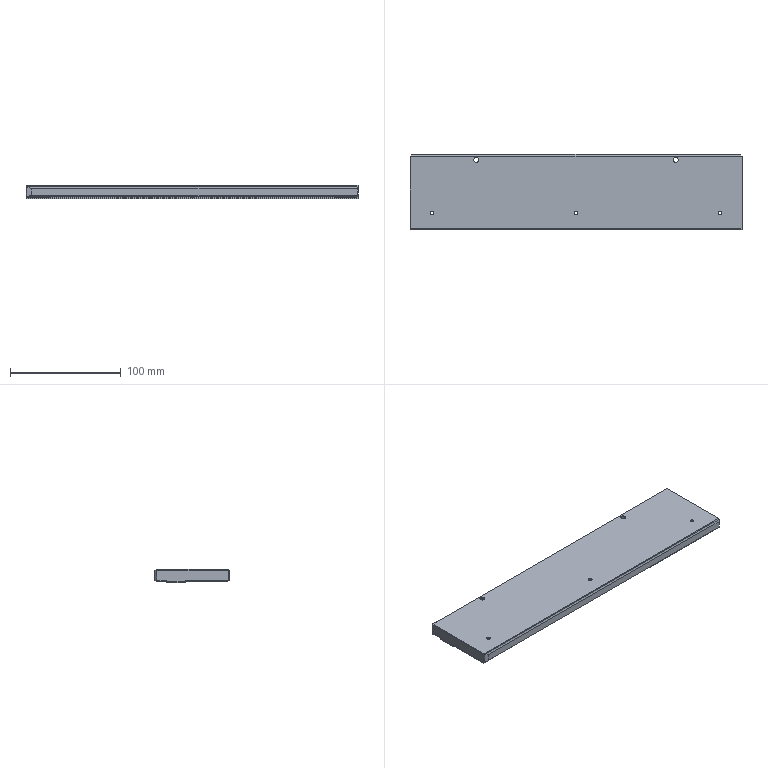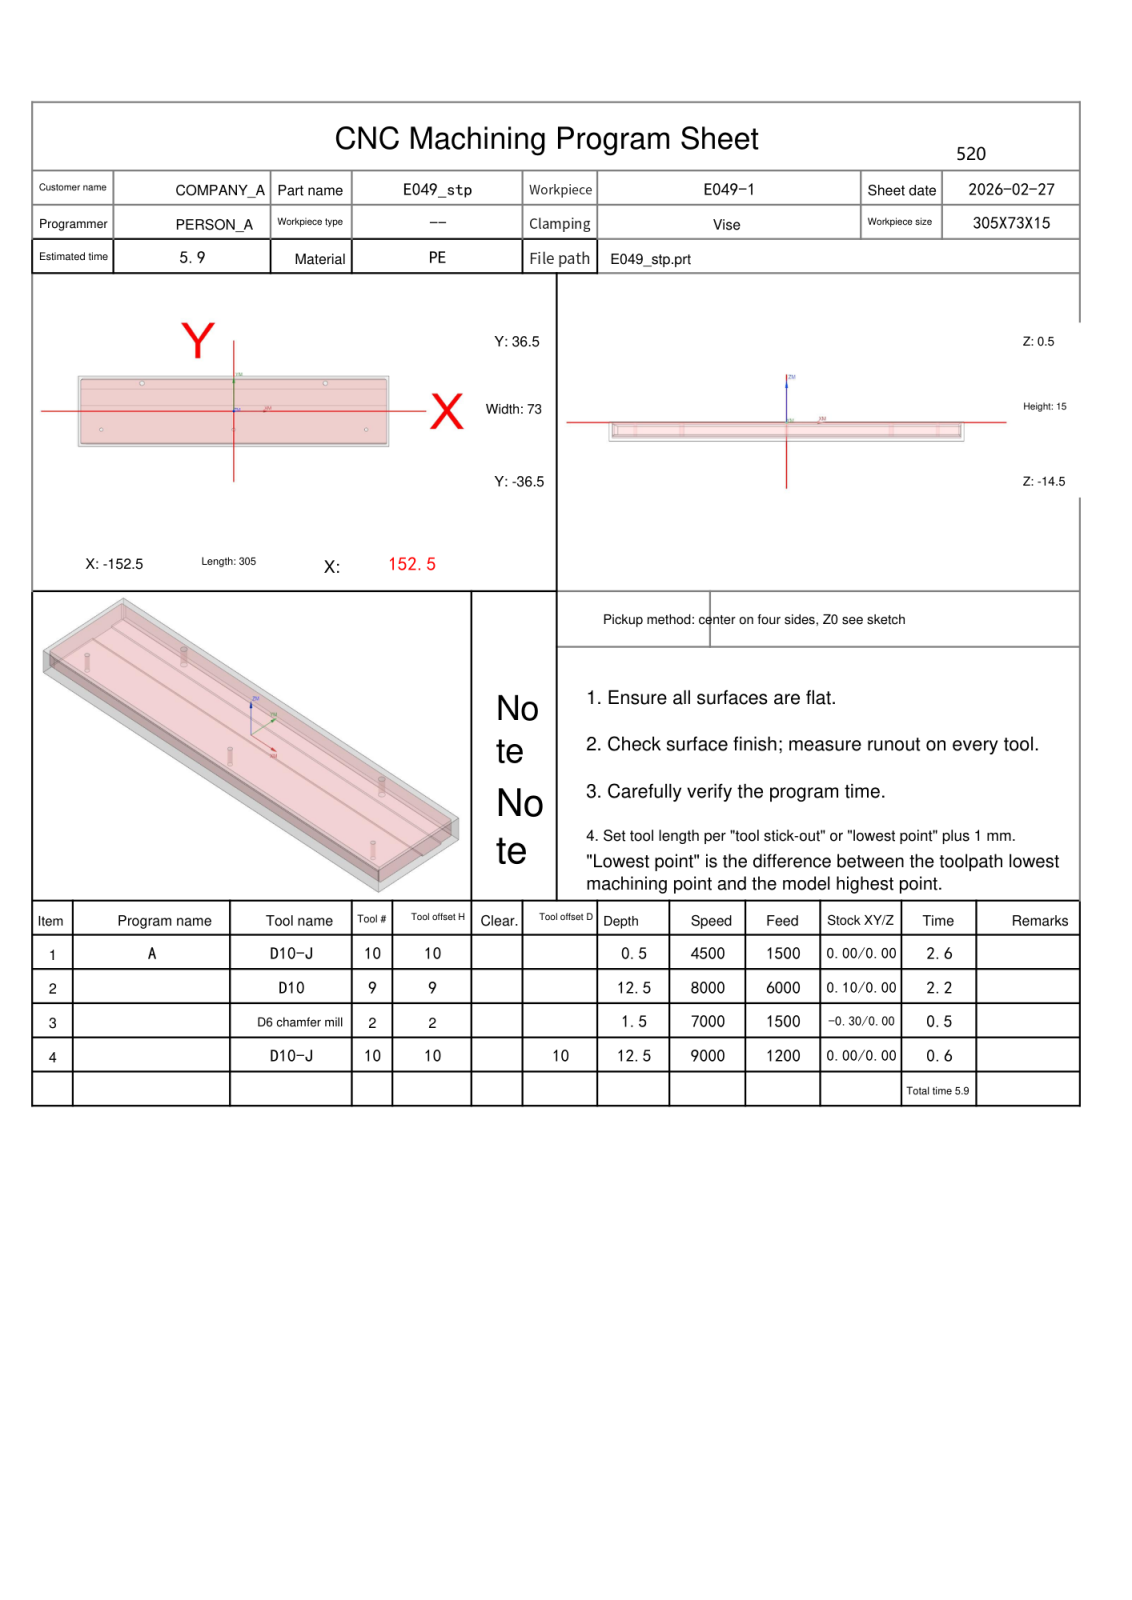NC program | NX | posted by the shop | part box 300 x 68 x 12 mm
Whole program:
%
O0001
(Machine time: 6.78 MIN)
(===Total Tool:3===)
(T10=D10-J  D=10.  R=0.   D-  H10 Z=-12.  )
(T9=D10     D=10.  R=0.   D-  H09 Z=-12.  )
(T2=D6 chamfer mill   D=6.   R=0.   D-  H02 Z=-1.   )
G80 G90 G17 G49 G40
G91 G28 Z0
M01
N1 T10 M06
(D10-J  D=10. R=0. H=10 ce=0.00 di=0.00)
G00 G90 G54 X-160. Y24.3 M03 S4500
G43 H10 Z30.
M08
Z2.
G01 Z0.0 F1500.
X-155. Y29.3
X-145.3 Y39.
X-135.6
X-155. Y19.6
Y9.9
X-125.9 Y39.
X-116.2
X-155. Y.2
Y-9.5
X-106.5 Y39.
X-96.8
X-155. Y-19.2
Y-28.9
X-87.1 Y39.
X-77.4
X-155. Y-38.6
Y-39.
X-145.7
X-67.7 Y39.
X-58.
X-136. Y-39.
X-126.3
X-48.3 Y39.
X-38.6
X-116.6 Y-39.
X-106.9
X-28.9 Y39.
X-19.2
X-97.2 Y-39.
X-87.5
X-9.5 Y39.
X.2
X-77.8 Y-39.
X-68.1
X9.9 Y39.
X19.6
X-58.4 Y-39.
X-48.7
X29.3 Y39.
X39.
X-39. Y-39.
X-29.3
X48.7 Y39.
X58.4
X-19.6 Y-39.
X-9.9
X68.1 Y39.
X77.8
X-.2 Y-39.
X9.5
X87.5 Y39.
X97.2
X19.2 Y-39.
X28.9
X106.9 Y39.
X116.6
X38.6 Y-39.
X48.3
X126.3 Y39.
X136.
X58. Y-39.
X67.7
X145.7 Y39.
X155.
Y38.6
X77.4 Y-39.
X87.1
X155. Y28.9
Y19.2
X96.8 Y-39.
X106.5
X155. Y9.5
Y-.2
X116.2 Y-39.
X125.9
X155. Y-9.9
Y-19.6
X135.6 Y-39.
X145.3
X155. Y-29.3
X160. Y-24.3
Z2.
G00 Z30.
G91 G28 Z0.0
M05
M09
G91 G28 Z0.0
M01
N2 T09 M06
(D10  D=10. R=0. H=09 ce=0.10 di=0.00)
G00 G90 G54 X-.267 Y-39.1 M03 S8000
G43 H09 Z30.
M08
Z.5
G01 X-145.254 Z.352 F6000.
X-150.01 Y-38.624 Z.347
G02 X-153.284 Y-36.972 Z.343 I.507 J5.075
G01 X-153.781 Y-36.422 Z.342
G02 X-155.1 Y-33. Z.339 I3.781 J3.422
G01 Y32. Z.272
G02 X-153.606 Y35.606 Z.268 I5.1 J0.0
G01 X-151.606 Y37.606 Z.265
G02 X-148. Y39.1 Z.261 I3.606 J-3.606
G01 X148. Z-.041
G02 X151.606 Y37.606 Z-.045 I0.0 J-5.1
G01 X153.606 Y35.606 Z-.048
G02 X155.1 Y32. Z-.052 I-3.606 J-3.606
G01 Y-33.5 Z-.119
G02 X153.606 Y-37.106 Z-.123 I-5.1 J0.0
G01 X153.106 Y-37.606 Z-.124
G02 X149.5 Y-39.1 Z-.128 I-3.606 J3.606
G01 X-145.254 Z-.429
X-150.01 Y-38.624 Z-.434
G02 X-153.284 Y-36.972 Z-.438 I.507 J5.075
G01 X-153.781 Y-36.422 Z-.439
G02 X-155.1 Y-33. Z-.443 I3.781 J3.422
G01 Y32. Z-.509
G02 X-153.606 Y35.606 Z-.513 I5.1 J0.0
G01 X-151.606 Y37.606 Z-.516
G02 X-148. Y39.1 Z-.52 I3.606 J-3.606
G01 X148. Z-.823
G02 X151.606 Y37.606 Z-.827 I0.0 J-5.1
G01 X153.606 Y35.606 Z-.83
G02 X155.1 Y32. Z-.834 I-3.606 J-3.606
G01 Y-33.5 Z-.901
G02 X153.606 Y-37.106 Z-.905 I-5.1 J0.0
G01 X153.106 Y-37.606
G02 X149.5 Y-39.1 Z-.909 I-3.606 J3.606
G01 X-145.254 Z-1.211
X-150.01 Y-38.624 Z-1.216
G02 X-153.284 Y-36.972 Z-1.219 I.507 J5.075
G01 X-153.781 Y-36.422 Z-1.22
G02 X-155.1 Y-33. Z-1.224 I3.781 J3.422
G01 Y32. Z-1.29
G02 X-153.606 Y35.606 Z-1.294 I5.1 J0.0
G01 X-151.606 Y37.606 Z-1.297
G02 X-148. Y39.1 Z-1.301 I3.606 J-3.606
G01 X148. Z-1.604
G02 X151.606 Y37.606 Z-1.608 I0.0 J-5.1
G01 X153.606 Y35.606 Z-1.611
G02 X155.1 Y32. Z-1.615 I-3.606 J-3.606
G01 Y-33.5 Z-1.682
G02 X153.606 Y-37.106 Z-1.686 I-5.1 J0.0
G01 X153.106 Y-37.606 Z-1.687
G02 X149.5 Y-39.1 Z-1.691 I-3.606 J3.606
G01 X-145.254 Z-1.992
X-150.01 Y-38.624 Z-1.997
G02 X-153.284 Y-36.972 Z-2.001 I.507 J5.075
G01 X-153.781 Y-36.422
G02 X-155.1 Y-33. Z-2.005 I3.781 J3.422
G01 Y32. Z-2.072
G02 X-153.606 Y35.606 Z-2.076 I5.1 J0.0
G01 X-151.606 Y37.606 Z-2.079
G02 X-148. Y39.1 Z-2.083 I3.606 J-3.606
G01 X148. Z-2.385
G02 X151.606 Y37.606 Z-2.389 I0.0 J-5.1
G01 X153.606 Y35.606 Z-2.392
G02 X155.1 Y32. Z-2.396 I-3.606 J-3.606
G01 Y-33.5 Z-2.463
G02 X153.606 Y-37.106 Z-2.467 I-5.1 J0.0
G01 X153.106 Y-37.606 Z-2.468
G02 X149.5 Y-39.1 Z-2.472 I-3.606 J3.606
G01 X-145.254 Z-2.773
X-150.01 Y-38.624 Z-2.778
G02 X-153.284 Y-36.972 Z-2.782 I.507 J5.075
G01 X-153.781 Y-36.422 Z-2.783
G02 X-155.1 Y-33. Z-2.786 I3.781 J3.422
G01 Y32. Z-2.853
G02 X-153.606 Y35.606 Z-2.857 I5.1 J0.0
G01 X-151.606 Y37.606 Z-2.86
G02 X-148. Y39.1 Z-2.864 I3.606 J-3.606
G01 X148. Z-3.166
G02 X151.606 Y37.606 Z-3.17 I0.0 J-5.1
G01 X153.606 Y35.606 Z-3.173
G02 X155.1 Y32. Z-3.177 I-3.606 J-3.606
G01 Y-33.5 Z-3.244
G02 X153.606 Y-37.106 Z-3.248 I-5.1 J0.0
G01 X153.106 Y-37.606 Z-3.249
G02 X149.5 Y-39.1 Z-3.253 I-3.606 J3.606
G01 X-145.254 Z-3.554
X-150.01 Y-38.624 Z-3.559
G02 X-153.284 Y-36.972 Z-3.563 I.507 J5.075
G01 X-153.781 Y-36.422 Z-3.564
G02 X-155.1 Y-33. Z-3.568 I3.781 J3.422
G01 Y32. Z-3.634
G02 X-153.606 Y35.606 Z-3.638 I5.1 J0.0
G01 X-151.606 Y37.606 Z-3.641
G02 X-148. Y39.1 Z-3.645 I3.606 J-3.606
G01 X148. Z-3.948
G02 X151.606 Y37.606 Z-3.952 I0.0 J-5.1
G01 X153.606 Y35.606 Z-3.955
G02 X155.1 Y32. Z-3.959 I-3.606 J-3.606
G01 Y-33.5 Z-4.026
G02 X153.606 Y-37.106 Z-4.03 I-5.1 J0.0
G01 X153.106 Y-37.606
G02 X149.5 Y-39.1 Z-4.034 I-3.606 J3.606
G01 X-145.254 Z-4.336
X-150.01 Y-38.624 Z-4.341
G02 X-153.284 Y-36.972 Z-4.344 I.507 J5.075
G01 X-153.781 Y-36.422 Z-4.345
G02 X-155.1 Y-33. Z-4.349 I3.781 J3.422
G01 Y32. Z-4.415
G02 X-153.606 Y35.606 Z-4.419 I5.1 J0.0
G01 X-151.606 Y37.606 Z-4.422
G02 X-148. Y39.1 Z-4.426 I3.606 J-3.606
G01 X148. Z-4.729
G02 X151.606 Y37.606 Z-4.733 I0.0 J-5.1
G01 X153.606 Y35.606 Z-4.736
G02 X155.1 Y32. Z-4.74 I-3.606 J-3.606
G01 Y-33.5 Z-4.807
G02 X153.606 Y-37.106 Z-4.811 I-5.1 J0.0
G01 X153.106 Y-37.606 Z-4.812
G02 X149.5 Y-39.1 Z-4.816 I-3.606 J3.606
G01 X-145.254 Z-5.117
X-150.01 Y-38.624 Z-5.122
G02 X-153.284 Y-36.972 Z-5.126 I.507 J5.075
G01 X-153.781 Y-36.422
G02 X-155.1 Y-33. Z-5.13 I3.781 J3.422
G01 Y32. Z-5.197
G02 X-153.606 Y35.606 Z-5.201 I5.1 J0.0
G01 X-151.606 Y37.606 Z-5.204
G02 X-148. Y39.1 Z-5.208 I3.606 J-3.606
G01 X148. Z-5.51
G02 X151.606 Y37.606 Z-5.514 I0.0 J-5.1
G01 X153.606 Y35.606 Z-5.517
G02 X155.1 Y32. Z-5.521 I-3.606 J-3.606
G01 Y-33.5 Z-5.588
G02 X153.606 Y-37.106 Z-5.592 I-5.1 J0.0
G01 X153.106 Y-37.606 Z-5.593
G02 X149.5 Y-39.1 Z-5.597 I-3.606 J3.606
G01 X-145.254 Z-5.898
X-150.01 Y-38.624 Z-5.903
G02 X-153.284 Y-36.972 Z-5.907 I.507 J5.075
G01 X-153.781 Y-36.422 Z-5.908
G02 X-155.1 Y-33. Z-5.911 I3.781 J3.422
G01 Y32. Z-5.978
G02 X-153.606 Y35.606 Z-5.982 I5.1 J0.0
G01 X-151.606 Y37.606 Z-5.985
G02 X-148. Y39.1 Z-5.989 I3.606 J-3.606
G01 X148. Z-6.291
G02 X151.606 Y37.606 Z-6.295 I0.0 J-5.1
G01 X153.606 Y35.606 Z-6.298
G02 X155.1 Y32. Z-6.302 I-3.606 J-3.606
G01 Y-33.5 Z-6.369
G02 X153.606 Y-37.106 Z-6.373 I-5.1 J0.0
G01 X153.106 Y-37.606 Z-6.374
G02 X149.5 Y-39.1 Z-6.378 I-3.606 J3.606
G01 X-145.254 Z-6.679
X-150.01 Y-38.624 Z-6.684
G02 X-153.284 Y-36.972 Z-6.688 I.507 J5.075
G01 X-153.781 Y-36.422 Z-6.689
G02 X-155.1 Y-33. Z-6.693 I3.781 J3.422
G01 Y32. Z-6.759
G02 X-153.606 Y35.606 Z-6.763 I5.1 J0.0
G01 X-151.606 Y37.606 Z-6.766
G02 X-148. Y39.1 Z-6.77 I3.606 J-3.606
G01 X148. Z-7.073
G02 X151.606 Y37.606 Z-7.077 I0.0 J-5.1
G01 X153.606 Y35.606 Z-7.08
G02 X155.1 Y32. Z-7.084 I-3.606 J-3.606
G01 Y-33.5 Z-7.151
G02 X153.606 Y-37.106 Z-7.155 I-5.1 J0.0
G01 X153.106 Y-37.606
G02 X149.5 Y-39.1 Z-7.159 I-3.606 J3.606
G01 X-145.254 Z-7.461
X-150.01 Y-38.624 Z-7.466
G02 X-153.284 Y-36.972 Z-7.469 I.507 J5.075
G01 X-153.781 Y-36.422 Z-7.47
G02 X-155.1 Y-33. Z-7.474 I3.781 J3.422
G01 Y32. Z-7.54
G02 X-153.606 Y35.606 Z-7.544 I5.1 J0.0
G01 X-151.606 Y37.606 Z-7.547
G02 X-148. Y39.1 Z-7.551 I3.606 J-3.606
G01 X148. Z-7.854
G02 X151.606 Y37.606 Z-7.858 I0.0 J-5.1
G01 X153.606 Y35.606 Z-7.861
G02 X155.1 Y32. Z-7.865 I-3.606 J-3.606
G01 Y-33.5 Z-7.932
G02 X153.606 Y-37.106 Z-7.936 I-5.1 J0.0
G01 X153.106 Y-37.606 Z-7.937
G02 X149.5 Y-39.1 Z-7.941 I-3.606 J3.606
G01 X-145.254 Z-8.242
X-150.01 Y-38.624 Z-8.247
G02 X-153.284 Y-36.972 Z-8.251 I.507 J5.075
G01 X-153.781 Y-36.422
G02 X-155.1 Y-33. Z-8.255 I3.781 J3.422
G01 Y32. Z-8.322
G02 X-153.606 Y35.606 Z-8.326 I5.1 J0.0
G01 X-151.606 Y37.606 Z-8.329
G02 X-148. Y39.1 Z-8.333 I3.606 J-3.606
G01 X148. Z-8.635
G02 X151.606 Y37.606 Z-8.639 I0.0 J-5.1
G01 X153.606 Y35.606 Z-8.642
G02 X155.1 Y32. Z-8.646 I-3.606 J-3.606
G01 Y-33.5 Z-8.713
G02 X153.606 Y-37.106 Z-8.717 I-5.1 J0.0
G01 X153.106 Y-37.606 Z-8.718
G02 X149.5 Y-39.1 Z-8.722 I-3.606 J3.606
G01 X-145.254 Z-9.023
X-150.01 Y-38.624 Z-9.028
G02 X-153.284 Y-36.972 Z-9.032 I.507 J5.075
G01 X-153.781 Y-36.422 Z-9.033
G02 X-155.1 Y-33. Z-9.036 I3.781 J3.422
G01 Y32. Z-9.103
G02 X-153.606 Y35.606 Z-9.107 I5.1 J0.0
G01 X-151.606 Y37.606 Z-9.11
G02 X-148. Y39.1 Z-9.114 I3.606 J-3.606
G01 X148. Z-9.416
G02 X151.606 Y37.606 Z-9.42 I0.0 J-5.1
G01 X153.606 Y35.606 Z-9.423
G02 X155.1 Y32. Z-9.427 I-3.606 J-3.606
G01 Y-33.5 Z-9.494
G02 X153.606 Y-37.106 Z-9.498 I-5.1 J0.0
G01 X153.106 Y-37.606 Z-9.499
G02 X149.5 Y-39.1 Z-9.503 I-3.606 J3.606
G01 X-145.254 Z-9.804
X-150.01 Y-38.624 Z-9.809
G02 X-153.284 Y-36.972 Z-9.813 I.507 J5.075
G01 X-153.781 Y-36.422 Z-9.814
G02 X-155.1 Y-33. Z-9.818 I3.781 J3.422
G01 Y32. Z-9.884
G02 X-153.606 Y35.606 Z-9.888 I5.1 J0.0
G01 X-151.606 Y37.606 Z-9.891
G02 X-148. Y39.1 Z-9.895 I3.606 J-3.606
G01 X148. Z-10.198
G02 X151.606 Y37.606 Z-10.202 I0.0 J-5.1
G01 X153.606 Y35.606 Z-10.205
G02 X155.1 Y32. Z-10.209 I-3.606 J-3.606
G01 Y-33.5 Z-10.276
G02 X153.606 Y-37.106 Z-10.28 I-5.1 J0.0
G01 X153.106 Y-37.606
G02 X149.5 Y-39.1 Z-10.284 I-3.606 J3.606
G01 X-145.254 Z-10.586
X-150.01 Y-38.624 Z-10.591
G02 X-153.284 Y-36.972 Z-10.594 I.507 J5.075
G01 X-153.781 Y-36.422 Z-10.595
G02 X-155.1 Y-33. Z-10.599 I3.781 J3.422
G01 Y32. Z-10.665
G02 X-153.606 Y35.606 Z-10.669 I5.1 J0.0
G01 X-151.606 Y37.606 Z-10.672
G02 X-148. Y39.1 Z-10.676 I3.606 J-3.606
G01 X148. Z-10.979
G02 X151.606 Y37.606 Z-10.983 I0.0 J-5.1
G01 X153.606 Y35.606 Z-10.986
G02 X155.1 Y32. Z-10.99 I-3.606 J-3.606
G01 Y-33.5 Z-11.057
G02 X153.606 Y-37.106 Z-11.061 I-5.1 J0.0
G01 X153.106 Y-37.606 Z-11.062
G02 X149.5 Y-39.1 Z-11.066 I-3.606 J3.606
G01 X-145.254 Z-11.367
X-150.01 Y-38.624 Z-11.372
G02 X-153.284 Y-36.972 Z-11.376 I.507 J5.075
G01 X-153.781 Y-36.422
G02 X-155.1 Y-33. Z-11.38 I3.781 J3.422
G01 Y32. Z-11.447
G02 X-153.606 Y35.606 Z-11.451 I5.1 J0.0
G01 X-151.606 Y37.606 Z-11.454
G02 X-148. Y39.1 Z-11.458 I3.606 J-3.606
G01 X148. Z-11.76
G02 X151.606 Y37.606 Z-11.764 I0.0 J-5.1
G01 X153.606 Y35.606 Z-11.767
G02 X155.1 Y32. Z-11.771 I-3.606 J-3.606
G01 Y-33.5 Z-11.838
G02 X153.606 Y-37.106 Z-11.842 I-5.1 J0.0
G01 X153.106 Y-37.606 Z-11.843
G02 X149.5 Y-39.1 Z-11.847 I-3.606 J3.606
G01 X-.267 Z-12.
X-145.254
X-150.01 Y-38.624
G02 X-153.284 Y-36.972 I.507 J5.075
G01 X-153.781 Y-36.422
G02 X-155.1 Y-33. I3.781 J3.422
G01 Y32.
G02 X-153.606 Y35.606 I5.1 J0.0
G01 X-151.606 Y37.606
G02 X-148. Y39.1 I3.606 J-3.606
G01 X148.
G02 X151.606 Y37.606 I0.0 J-5.1
G01 X153.606 Y35.606
G02 X155.1 Y32. I-3.606 J-3.606
G01 Y-33.5
G02 X153.606 Y-37.106 I-5.1 J0.0
G01 X153.106 Y-37.606
G02 X149.5 Y-39.1 I-3.606 J3.606
G01 X-.267
X-.767
Z-11.
G00 Z30.
G91 G28 Z0.0
M05
M09
G91 G28 Z0.0
M01
N3 T02 M06
(D6 chamfer mill  D=6. R=0. H=02 ce=-0.30 di=0.00)
G00 G90 G54 X-141.847 Y-34.7 M03 S7000
G43 H02 Z30.
M08
Z2.5
G01 X-144.985 Z1.358 F1500.
X-145.035 Z1.34
X-149.534 Y-34.25 Z-.306
X-149.721 Y-34.198 Z-.377
X-149.894 Y-34.11 Z-.447
X-150.047 Y-33.991 Z-.518
X-150.493 Y-33.498 Z-.76
X-150.597 Y-33.334 Z-.831
X-150.666 Y-33.153 Z-.901
X-150.7 Y-32.962 Z-.972
Y-32.884 Z-1.
Y31.876
G02 X-150.407 Y32.583 I1. J0.0
G01 X-148.583 Y34.407
G02 X-147.876 Y34.7 I.707 J-.707
G01 X147.876
G02 X148.583 Y34.407 I0.0 J-1.
G01 X150.407 Y32.583
G02 X150.7 Y31.876 I-.707 J-.707
G01 Y-33.376
G02 X150.407 Y-34.083 I-1. J0.0
G01 X150.083 Y-34.407
G02 X149.376 Y-34.7 I-.707 J.707
G01 X-144.985
X-145.035 Y-34.702
X-145.085 Y-34.695
X-149.457 Y-34.258
G02 X-150.099 Y-33.934 I.1 J.995
G01 X-150.441 Y-33.555
G02 X-150.7 Y-32.884 I.741 J.671
G01 Y-32.384
Z1.5
G00 Z30.
G91 G28 Z0.0
M05
M09
G91 G28 Z0.0
M01
N4 T10 M06
(D10-J  D=10. R=0. H=10 ce=0.00 di=0.00)
G00 G90 G54 X150.513 Y-40.116 M03 S9000
G43 H10 Z30.
M08
Z-11.5
G01 Z-12. F1200.
G41 D10
X150.497 Y-39.917
G03 X149.5 Y-39. I-.997 J-.083
G01 X-145.249
X-150. Y-38.525
G02 X-153.21 Y-36.905 I.498 J4.975
G01 X-153.707 Y-36.355
G02 X-155. Y-33. I3.707 J3.355
G01 Y32.
G02 X-153.536 Y35.536 I5. J0.0
G01 X-151.536 Y37.536
G02 X-148. Y39. I3.536 J-3.536
G01 X148.
G02 X151.536 Y37.536 I0.0 J-5.
G01 X153.536 Y35.536
G02 X155. Y32. I-3.536 J-3.536
G01 Y-33.5
G02 X153.536 Y-37.036 I-5. J0.0
G01 X153.036 Y-37.536
G02 X149.5 Y-39. I-3.536 J3.536
G01 X149.
G03 X148. Y-40. I0.0 J-1.
G01 G40 Y-40.2
Z-11.5
G00 Z30.
M05
M09
G91 G28 Z0.0
G91 G28 Y0.0
M30
%